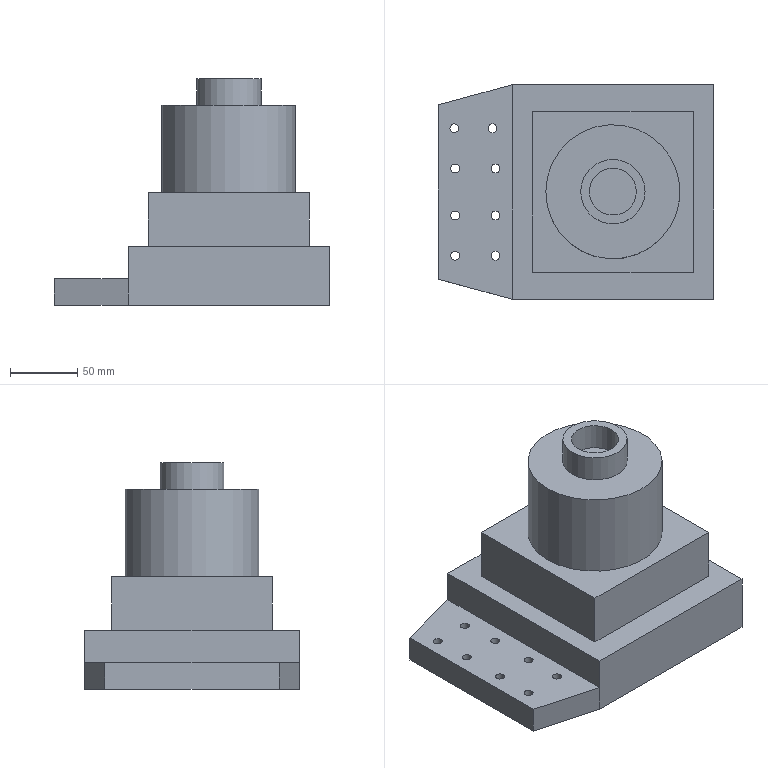Part | STEP file | PROJECTION BASE 1 WASHER | 1 solid | 29 faces | box 205 x 160 x 169 mm | volume 2313406 mm3 | plane 18 | cylinder 11 | commonest cylinder face diameters 6.647 x8 35 x1 48 x1 100 x1